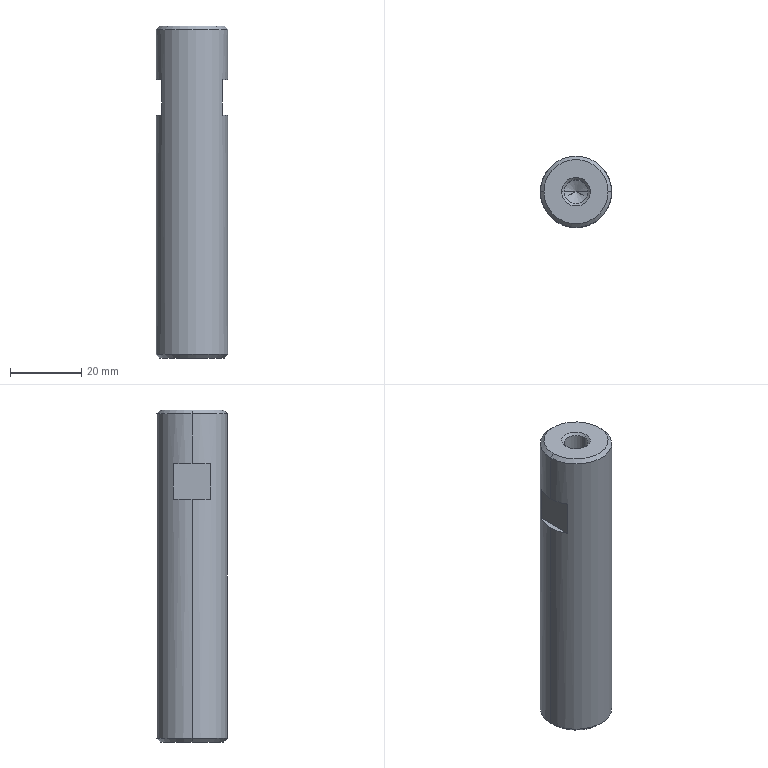Part | NX | features BREP 1 | 1 solid | 26 faces | box 20 x 20 x 93 mm | volume 27742 mm3 | cone 12 | plane 8 | cylinder 6 | commonest cylinder face diameters 6.647 x4 20 x2
STEP:
#1=CARTESIAN_POINT('',(3.324,0.,-92.323));
#2=VERTEX_POINT('',#1);
#3=CARTESIAN_POINT('',(-3.324,0.,-92.323));
#4=VERTEX_POINT('',#3);
#5=CARTESIAN_POINT('',(0.,0.,-92.323));
#6=DIRECTION('',(0.,0.,-1.));
#7=DIRECTION('',(-1.,0.,0.));
#8=AXIS2_PLACEMENT_3D('',#5,#6,#7);
#9=CIRCLE('',#8,3.324);
#10=EDGE_CURVE('',#2,#4,#9,.T.);
#11=ORIENTED_EDGE('',*,*,#10,.F.);
#12=CARTESIAN_POINT('',(4.,0.,-93.));
#13=VERTEX_POINT('',#12);
#14=CARTESIAN_POINT('',(4.,0.,-93.));
#15=DIRECTION('',(0.7071,0.,-0.7071));
#16=VECTOR('',#15,1000.);
#17=LINE('',#14,#16);
#18=EDGE_CURVE('',#13,#2,#17,.F.);
#19=ORIENTED_EDGE('',*,*,#18,.F.);
#20=CARTESIAN_POINT('',(-4.,0.,-93.));
#21=VERTEX_POINT('',#20);
#22=CARTESIAN_POINT('',(0.,0.,-93.));
#23=DIRECTION('',(0.,0.,-1.));
#24=DIRECTION('',(-1.,0.,0.));
#25=AXIS2_PLACEMENT_3D('',#22,#23,#24);
#26=CIRCLE('',#25,4.);
#27=EDGE_CURVE('',#13,#21,#26,.T.);
#28=ORIENTED_EDGE('',*,*,#27,.T.);
#29=CARTESIAN_POINT('',(-4.,0.,-93.));
#30=DIRECTION('',(-0.7071,0.,-0.7071));
#31=VECTOR('',#30,1000.);
#32=LINE('',#29,#31);
#33=EDGE_CURVE('',#21,#4,#32,.F.);
#34=ORIENTED_EDGE('',*,*,#33,.T.);
#35=EDGE_LOOP('',(#11,#19,#28,#34));
#36=FACE_BOUND('',#35,.T.);
#37=CARTESIAN_POINT('',(0.,0.,-93.));
#38=DIRECTION('',(0.,0.,-1.));
#39=DIRECTION('',(1.,0.,0.));
#40=AXIS2_PLACEMENT_3D('',#37,#38,#39);
#41=CONICAL_SURFACE('',#40,4.,0.7854);
#42=ADVANCED_FACE('',(#36),#41,.F.);
#43=CARTESIAN_POINT('',(3.324,0.,-76.5));
#44=VERTEX_POINT('',#43);
#45=CARTESIAN_POINT('',(-3.324,0.,-76.5));
#46=VERTEX_POINT('',#45);
#47=CARTESIAN_POINT('',(0.,0.,-76.5));
#48=DIRECTION('',(0.,0.,-1.));
#49=DIRECTION('',(-1.,0.,0.));
#50=AXIS2_PLACEMENT_3D('',#47,#48,#49);
#51=CIRCLE('',#50,3.324);
#52=EDGE_CURVE('',#44,#46,#51,.T.);
#53=ORIENTED_EDGE('',*,*,#52,.F.);
#54=CARTESIAN_POINT('',(3.324,0.,-93.));
#55=DIRECTION('',(0.,0.,-1.));
#56=VECTOR('',#55,1000.);
#57=LINE('',#54,#56);
#58=EDGE_CURVE('',#2,#44,#57,.F.);
#59=ORIENTED_EDGE('',*,*,#58,.F.);
#60=ORIENTED_EDGE('',*,*,#10,.T.);
#61=CARTESIAN_POINT('',(-3.324,0.,-93.));
#62=DIRECTION('',(0.,0.,-1.));
#63=VECTOR('',#62,1000.);
#64=LINE('',#61,#63);
#65=EDGE_CURVE('',#4,#46,#64,.F.);
#66=ORIENTED_EDGE('',*,*,#65,.T.);
#67=EDGE_LOOP('',(#53,#59,#60,#66));
#68=FACE_BOUND('',#67,.T.);
#69=CARTESIAN_POINT('',(0.,0.,-93.));
#70=DIRECTION('',(0.,0.,-1.));
#71=DIRECTION('',(1.,0.,0.));
#72=AXIS2_PLACEMENT_3D('',#69,#70,#71);
#73=CYLINDRICAL_SURFACE('',#72,3.324);
#74=ADVANCED_FACE('',(#68),#73,.F.);
#75=CARTESIAN_POINT('',(0.,0.,-74.581));
#76=VERTEX_POINT('',#75);
#77=CARTESIAN_POINT('',(-3.324,0.,-76.5));
#78=DIRECTION('',(-0.866,0.,-0.5));
#79=VECTOR('',#78,1000.);
#80=LINE('',#77,#79);
#81=EDGE_CURVE('',#46,#76,#80,.F.);
#82=ORIENTED_EDGE('',*,*,#81,.T.);
#83=CARTESIAN_POINT('',(3.324,0.,-76.5));
#84=DIRECTION('',(0.866,0.,-0.5));
#85=VECTOR('',#84,1000.);
#86=LINE('',#83,#85);
#87=EDGE_CURVE('',#44,#76,#86,.F.);
#88=ORIENTED_EDGE('',*,*,#87,.F.);
#89=ORIENTED_EDGE('',*,*,#52,.T.);
#90=EDGE_LOOP('',(#82,#88,#89));
#91=FACE_BOUND('',#90,.T.);
#92=CARTESIAN_POINT('',(0.,0.,-76.5));
#93=DIRECTION('',(0.,0.,-1.));
#94=DIRECTION('',(1.,0.,0.));
#95=AXIS2_PLACEMENT_3D('',#92,#93,#94);
#96=CONICAL_SURFACE('',#95,3.324,1.047);
#97=ADVANCED_FACE('',(#91),#96,.F.);
#98=CARTESIAN_POINT('',(-3.324,0.,-0.6765));
#99=VERTEX_POINT('',#98);
#100=CARTESIAN_POINT('',(3.324,0.,-0.6765));
#101=VERTEX_POINT('',#100);
#102=CARTESIAN_POINT('',(0.,0.,-0.6765));
#103=DIRECTION('',(0.,0.,1.));
#104=DIRECTION('',(1.,0.,0.));
#105=AXIS2_PLACEMENT_3D('',#102,#103,#104);
#106=CIRCLE('',#105,3.324);
#107=EDGE_CURVE('',#99,#101,#106,.T.);
#108=ORIENTED_EDGE('',*,*,#107,.F.);
#109=CARTESIAN_POINT('',(-4.,0.,0.));
#110=VERTEX_POINT('',#109);
#111=CARTESIAN_POINT('',(-4.,0.,0.));
#112=DIRECTION('',(-0.7071,0.,0.7071));
#113=VECTOR('',#112,1000.);
#114=LINE('',#111,#113);
#115=EDGE_CURVE('',#99,#110,#114,.T.);
#116=ORIENTED_EDGE('',*,*,#115,.T.);
#117=CARTESIAN_POINT('',(4.,0.,0.));
#118=VERTEX_POINT('',#117);
#119=CARTESIAN_POINT('',(0.,0.,0.));
#120=DIRECTION('',(0.,0.,1.));
#121=DIRECTION('',(1.,0.,0.));
#122=AXIS2_PLACEMENT_3D('',#119,#120,#121);
#123=CIRCLE('',#122,4.);
#124=EDGE_CURVE('',#110,#118,#123,.T.);
#125=ORIENTED_EDGE('',*,*,#124,.T.);
#126=CARTESIAN_POINT('',(4.,0.,0.));
#127=DIRECTION('',(0.7071,0.,0.7071));
#128=VECTOR('',#127,1000.);
#129=LINE('',#126,#128);
#130=EDGE_CURVE('',#101,#118,#129,.T.);
#131=ORIENTED_EDGE('',*,*,#130,.F.);
#132=EDGE_LOOP('',(#108,#116,#125,#131));
#133=FACE_BOUND('',#132,.T.);
#134=CARTESIAN_POINT('',(0.,0.,0.));
#135=DIRECTION('',(0.,0.,1.));
#136=DIRECTION('',(-1.,0.,0.));
#137=AXIS2_PLACEMENT_3D('',#134,#135,#136);
#138=CONICAL_SURFACE('',#137,4.,0.7854);
#139=ADVANCED_FACE('',(#133),#138,.F.);
#140=CARTESIAN_POINT('',(-3.324,0.,-16.5));
#141=VERTEX_POINT('',#140);
#142=CARTESIAN_POINT('',(3.324,0.,-16.5));
#143=VERTEX_POINT('',#142);
#144=CARTESIAN_POINT('',(0.,0.,-16.5));
#145=DIRECTION('',(0.,0.,1.));
#146=DIRECTION('',(1.,0.,0.));
#147=AXIS2_PLACEMENT_3D('',#144,#145,#146);
#148=CIRCLE('',#147,3.324);
#149=EDGE_CURVE('',#141,#143,#148,.T.);
#150=ORIENTED_EDGE('',*,*,#149,.F.);
#151=CARTESIAN_POINT('',(-3.324,0.,0.));
#152=DIRECTION('',(0.,0.,1.));
#153=VECTOR('',#152,1000.);
#154=LINE('',#151,#153);
#155=EDGE_CURVE('',#141,#99,#154,.T.);
#156=ORIENTED_EDGE('',*,*,#155,.T.);
#157=ORIENTED_EDGE('',*,*,#107,.T.);
#158=CARTESIAN_POINT('',(3.324,0.,0.));
#159=DIRECTION('',(0.,0.,1.));
#160=VECTOR('',#159,1000.);
#161=LINE('',#158,#160);
#162=EDGE_CURVE('',#143,#101,#161,.T.);
#163=ORIENTED_EDGE('',*,*,#162,.F.);
#164=EDGE_LOOP('',(#150,#156,#157,#163));
#165=FACE_BOUND('',#164,.T.);
#166=CARTESIAN_POINT('',(0.,0.,0.));
#167=DIRECTION('',(0.,0.,1.));
#168=DIRECTION('',(-1.,0.,0.));
#169=AXIS2_PLACEMENT_3D('',#166,#167,#168);
#170=CYLINDRICAL_SURFACE('',#169,3.324);
#171=ADVANCED_FACE('',(#165),#170,.F.);
#172=CARTESIAN_POINT('',(0.,0.,-18.419));
#173=VERTEX_POINT('',#172);
#174=CARTESIAN_POINT('',(3.324,0.,-16.5));
#175=DIRECTION('',(0.866,0.,0.5));
#176=VECTOR('',#175,1000.);
#177=LINE('',#174,#176);
#178=EDGE_CURVE('',#173,#143,#177,.T.);
#179=ORIENTED_EDGE('',*,*,#178,.F.);
#180=CARTESIAN_POINT('',(-3.324,0.,-16.5));
#181=DIRECTION('',(-0.866,0.,0.5));
#182=VECTOR('',#181,1000.);
#183=LINE('',#180,#182);
#184=EDGE_CURVE('',#173,#141,#183,.T.);
#185=ORIENTED_EDGE('',*,*,#184,.T.);
#186=ORIENTED_EDGE('',*,*,#149,.T.);
#187=EDGE_LOOP('',(#179,#185,#186));
#188=FACE_BOUND('',#187,.T.);
#189=CARTESIAN_POINT('',(0.,0.,-16.5));
#190=DIRECTION('',(0.,0.,1.));
#191=DIRECTION('',(-1.,0.,0.));
#192=AXIS2_PLACEMENT_3D('',#189,#190,#191);
#193=CONICAL_SURFACE('',#192,3.324,1.047);
#194=ADVANCED_FACE('',(#188),#193,.F.);
#195=CARTESIAN_POINT('',(9.,0.,-93.));
#196=VERTEX_POINT('',#195);
#197=CARTESIAN_POINT('',(-9.,0.,-93.));
#198=VERTEX_POINT('',#197);
#199=CARTESIAN_POINT('',(0.,0.,-93.));
#200=DIRECTION('',(0.,0.,1.));
#201=DIRECTION('',(1.,0.,0.));
#202=AXIS2_PLACEMENT_3D('',#199,#200,#201);
#203=CIRCLE('',#202,9.);
#204=EDGE_CURVE('',#196,#198,#203,.T.);
#205=ORIENTED_EDGE('',*,*,#204,.T.);
#206=CARTESIAN_POINT('',(-10.,0.,-92.));
#207=VERTEX_POINT('',#206);
#208=CARTESIAN_POINT('',(-9.,0.,-93.));
#209=DIRECTION('',(-0.7071,0.,0.7071));
#210=VECTOR('',#209,1000.);
#211=LINE('',#208,#210);
#212=EDGE_CURVE('',#198,#207,#211,.T.);
#213=ORIENTED_EDGE('',*,*,#212,.T.);
#214=CARTESIAN_POINT('',(10.,0.,-92.));
#215=VERTEX_POINT('',#214);
#216=CARTESIAN_POINT('',(0.,0.,-92.));
#217=DIRECTION('',(0.,0.,1.));
#218=DIRECTION('',(1.,0.,0.));
#219=AXIS2_PLACEMENT_3D('',#216,#217,#218);
#220=CIRCLE('',#219,10.);
#221=EDGE_CURVE('',#215,#207,#220,.T.);
#222=ORIENTED_EDGE('',*,*,#221,.F.);
#223=CARTESIAN_POINT('',(9.,0.,-93.));
#224=DIRECTION('',(0.7071,0.,0.7071));
#225=VECTOR('',#224,1000.);
#226=LINE('',#223,#225);
#227=EDGE_CURVE('',#196,#215,#226,.T.);
#228=ORIENTED_EDGE('',*,*,#227,.F.);
#229=EDGE_LOOP('',(#205,#213,#222,#228));
#230=FACE_BOUND('',#229,.T.);
#231=CARTESIAN_POINT('',(0.,0.,-93.));
#232=DIRECTION('',(0.,0.,1.));
#233=DIRECTION('',(-1.,0.,0.));
#234=AXIS2_PLACEMENT_3D('',#231,#232,#233);
#235=CONICAL_SURFACE('',#234,9.,0.7854);
#236=ADVANCED_FACE('',(#230),#235,.T.);
#237=CARTESIAN_POINT('',(9.,0.,0.));
#238=VERTEX_POINT('',#237);
#239=CARTESIAN_POINT('',(-9.,0.,0.));
#240=VERTEX_POINT('',#239);
#241=CARTESIAN_POINT('',(0.,0.,0.));
#242=DIRECTION('',(0.,0.,1.));
#243=DIRECTION('',(1.,0.,0.));
#244=AXIS2_PLACEMENT_3D('',#241,#242,#243);
#245=CIRCLE('',#244,9.);
#246=EDGE_CURVE('',#238,#240,#245,.T.);
#247=ORIENTED_EDGE('',*,*,#246,.F.);
#248=CARTESIAN_POINT('',(10.,0.,-1.));
#249=VERTEX_POINT('',#248);
#250=CARTESIAN_POINT('',(10.,0.,-1.));
#251=DIRECTION('',(0.7071,0.,-0.7071));
#252=VECTOR('',#251,1000.);
#253=LINE('',#250,#252);
#254=EDGE_CURVE('',#249,#238,#253,.F.);
#255=ORIENTED_EDGE('',*,*,#254,.F.);
#256=CARTESIAN_POINT('',(-10.,0.,-1.));
#257=VERTEX_POINT('',#256);
#258=CARTESIAN_POINT('',(0.,0.,-1.));
#259=DIRECTION('',(0.,0.,1.));
#260=DIRECTION('',(1.,0.,0.));
#261=AXIS2_PLACEMENT_3D('',#258,#259,#260);
#262=CIRCLE('',#261,10.);
#263=EDGE_CURVE('',#249,#257,#262,.T.);
#264=ORIENTED_EDGE('',*,*,#263,.T.);
#265=CARTESIAN_POINT('',(-10.,0.,-1.));
#266=DIRECTION('',(-0.7071,0.,-0.7071));
#267=VECTOR('',#266,1000.);
#268=LINE('',#265,#267);
#269=EDGE_CURVE('',#257,#240,#268,.F.);
#270=ORIENTED_EDGE('',*,*,#269,.T.);
#271=EDGE_LOOP('',(#247,#255,#264,#270));
#272=FACE_BOUND('',#271,.T.);
#273=CARTESIAN_POINT('',(0.,0.,-1.));
#274=DIRECTION('',(0.,0.,-1.));
#275=DIRECTION('',(1.,0.,0.));
#276=AXIS2_PLACEMENT_3D('',#273,#274,#275);
#277=CONICAL_SURFACE('',#276,10.,0.7854);
#278=ADVANCED_FACE('',(#272),#277,.T.);
#279=ORIENTED_EDGE('',*,*,#221,.T.);
#280=CARTESIAN_POINT('',(-10.,0.,-25.));
#281=VERTEX_POINT('',#280);
#282=CARTESIAN_POINT('',(-10.,0.,-93.));
#283=DIRECTION('',(0.,0.,1.));
#284=VECTOR('',#283,1000.);
#285=LINE('',#282,#284);
#286=EDGE_CURVE('',#207,#281,#285,.T.);
#287=ORIENTED_EDGE('',*,*,#286,.T.);
#288=CARTESIAN_POINT('',(-8.5,5.268,-25.));
#289=VERTEX_POINT('',#288);
#290=CARTESIAN_POINT('',(0.,0.,-25.));
#291=DIRECTION('',(0.,0.,1.));
#292=DIRECTION('',(1.,0.,0.));
#293=AXIS2_PLACEMENT_3D('',#290,#291,#292);
#294=CIRCLE('',#293,10.);
#295=EDGE_CURVE('',#289,#281,#294,.T.);
#296=ORIENTED_EDGE('',*,*,#295,.F.);
#297=CARTESIAN_POINT('',(-8.5,5.268,-15.));
#298=VERTEX_POINT('',#297);
#299=CARTESIAN_POINT('',(-8.5,5.268,-25.));
#300=DIRECTION('',(0.,0.,1.));
#301=VECTOR('',#300,1000.);
#302=LINE('',#299,#301);
#303=EDGE_CURVE('',#289,#298,#302,.T.);
#304=ORIENTED_EDGE('',*,*,#303,.T.);
#305=CARTESIAN_POINT('',(-10.,0.,-15.));
#306=VERTEX_POINT('',#305);
#307=CARTESIAN_POINT('',(0.,0.,-15.));
#308=DIRECTION('',(0.,0.,1.));
#309=DIRECTION('',(1.,0.,0.));
#310=AXIS2_PLACEMENT_3D('',#307,#308,#309);
#311=CIRCLE('',#310,10.);
#312=EDGE_CURVE('',#298,#306,#311,.T.);
#313=ORIENTED_EDGE('',*,*,#312,.T.);
#314=CARTESIAN_POINT('',(-10.,0.,-93.));
#315=DIRECTION('',(0.,0.,1.));
#316=VECTOR('',#315,1000.);
#317=LINE('',#314,#316);
#318=EDGE_CURVE('',#306,#257,#317,.T.);
#319=ORIENTED_EDGE('',*,*,#318,.T.);
#320=ORIENTED_EDGE('',*,*,#263,.F.);
#321=CARTESIAN_POINT('',(10.,0.,-15.));
#322=VERTEX_POINT('',#321);
#323=CARTESIAN_POINT('',(10.,0.,-93.));
#324=DIRECTION('',(0.,0.,1.));
#325=VECTOR('',#324,1000.);
#326=LINE('',#323,#325);
#327=EDGE_CURVE('',#322,#249,#326,.T.);
#328=ORIENTED_EDGE('',*,*,#327,.F.);
#329=CARTESIAN_POINT('',(8.5,5.268,-15.));
#330=VERTEX_POINT('',#329);
#331=CARTESIAN_POINT('',(0.,0.,-15.));
#332=DIRECTION('',(0.,0.,1.));
#333=DIRECTION('',(1.,0.,0.));
#334=AXIS2_PLACEMENT_3D('',#331,#332,#333);
#335=CIRCLE('',#334,10.);
#336=EDGE_CURVE('',#322,#330,#335,.T.);
#337=ORIENTED_EDGE('',*,*,#336,.T.);
#338=CARTESIAN_POINT('',(8.5,5.268,-25.));
#339=VERTEX_POINT('',#338);
#340=CARTESIAN_POINT('',(8.5,5.268,-25.));
#341=DIRECTION('',(0.,0.,1.));
#342=VECTOR('',#341,1000.);
#343=LINE('',#340,#342);
#344=EDGE_CURVE('',#339,#330,#343,.T.);
#345=ORIENTED_EDGE('',*,*,#344,.F.);
#346=CARTESIAN_POINT('',(10.,0.,-25.));
#347=VERTEX_POINT('',#346);
#348=CARTESIAN_POINT('',(0.,0.,-25.));
#349=DIRECTION('',(0.,0.,1.));
#350=DIRECTION('',(1.,0.,0.));
#351=AXIS2_PLACEMENT_3D('',#348,#349,#350);
#352=CIRCLE('',#351,10.);
#353=EDGE_CURVE('',#347,#339,#352,.T.);
#354=ORIENTED_EDGE('',*,*,#353,.F.);
#355=CARTESIAN_POINT('',(10.,0.,-93.));
#356=DIRECTION('',(0.,0.,1.));
#357=VECTOR('',#356,1000.);
#358=LINE('',#355,#357);
#359=EDGE_CURVE('',#215,#347,#358,.T.);
#360=ORIENTED_EDGE('',*,*,#359,.F.);
#361=EDGE_LOOP('',(#279,#287,#296,#304,#313,#319,#320,#328,#337,#345,#354,#360));
#362=FACE_BOUND('',#361,.T.);
#363=CARTESIAN_POINT('',(0.,0.,-93.));
#364=DIRECTION('',(0.,0.,1.));
#365=DIRECTION('',(-1.,0.,0.));
#366=AXIS2_PLACEMENT_3D('',#363,#364,#365);
#367=CYLINDRICAL_SURFACE('',#366,10.);
#368=ADVANCED_FACE('',(#362),#367,.T.);
#369=ORIENTED_EDGE('',*,*,#286,.F.);
#370=CARTESIAN_POINT('',(0.,0.,-92.));
#371=DIRECTION('',(0.,0.,1.));
#372=DIRECTION('',(1.,0.,0.));
#373=AXIS2_PLACEMENT_3D('',#370,#371,#372);
#374=CIRCLE('',#373,10.);
#375=EDGE_CURVE('',#207,#215,#374,.T.);
#376=ORIENTED_EDGE('',*,*,#375,.T.);
#377=ORIENTED_EDGE('',*,*,#359,.T.);
#378=CARTESIAN_POINT('',(8.5,-5.268,-25.));
#379=VERTEX_POINT('',#378);
#380=CARTESIAN_POINT('',(0.,0.,-25.));
#381=DIRECTION('',(0.,0.,1.));
#382=DIRECTION('',(1.,0.,0.));
#383=AXIS2_PLACEMENT_3D('',#380,#381,#382);
#384=CIRCLE('',#383,10.);
#385=EDGE_CURVE('',#379,#347,#384,.T.);
#386=ORIENTED_EDGE('',*,*,#385,.F.);
#387=CARTESIAN_POINT('',(8.5,-5.268,-15.));
#388=VERTEX_POINT('',#387);
#389=CARTESIAN_POINT('',(8.5,-5.268,-25.));
#390=DIRECTION('',(0.,0.,1.));
#391=VECTOR('',#390,1000.);
#392=LINE('',#389,#391);
#393=EDGE_CURVE('',#379,#388,#392,.T.);
#394=ORIENTED_EDGE('',*,*,#393,.T.);
#395=CARTESIAN_POINT('',(0.,0.,-15.));
#396=DIRECTION('',(0.,0.,1.));
#397=DIRECTION('',(1.,0.,0.));
#398=AXIS2_PLACEMENT_3D('',#395,#396,#397);
#399=CIRCLE('',#398,10.);
#400=EDGE_CURVE('',#388,#322,#399,.T.);
#401=ORIENTED_EDGE('',*,*,#400,.T.);
#402=ORIENTED_EDGE('',*,*,#327,.T.);
#403=CARTESIAN_POINT('',(0.,0.,-1.));
#404=DIRECTION('',(0.,0.,1.));
#405=DIRECTION('',(1.,0.,0.));
#406=AXIS2_PLACEMENT_3D('',#403,#404,#405);
#407=CIRCLE('',#406,10.);
#408=EDGE_CURVE('',#257,#249,#407,.T.);
#409=ORIENTED_EDGE('',*,*,#408,.F.);
#410=ORIENTED_EDGE('',*,*,#318,.F.);
#411=CARTESIAN_POINT('',(-8.5,-5.268,-15.));
#412=VERTEX_POINT('',#411);
#413=CARTESIAN_POINT('',(0.,0.,-15.));
#414=DIRECTION('',(0.,0.,1.));
#415=DIRECTION('',(1.,0.,0.));
#416=AXIS2_PLACEMENT_3D('',#413,#414,#415);
#417=CIRCLE('',#416,10.);
#418=EDGE_CURVE('',#306,#412,#417,.T.);
#419=ORIENTED_EDGE('',*,*,#418,.T.);
#420=CARTESIAN_POINT('',(-8.5,-5.268,-25.));
#421=VERTEX_POINT('',#420);
#422=CARTESIAN_POINT('',(-8.5,-5.268,-25.));
#423=DIRECTION('',(0.,0.,1.));
#424=VECTOR('',#423,1000.);
#425=LINE('',#422,#424);
#426=EDGE_CURVE('',#421,#412,#425,.T.);
#427=ORIENTED_EDGE('',*,*,#426,.F.);
#428=CARTESIAN_POINT('',(0.,0.,-25.));
#429=DIRECTION('',(0.,0.,1.));
#430=DIRECTION('',(1.,0.,0.));
#431=AXIS2_PLACEMENT_3D('',#428,#429,#430);
#432=CIRCLE('',#431,10.);
#433=EDGE_CURVE('',#281,#421,#432,.T.);
#434=ORIENTED_EDGE('',*,*,#433,.F.);
#435=EDGE_LOOP('',(#369,#376,#377,#386,#394,#401,#402,#409,#410,#419,#427,#434));
#436=FACE_BOUND('',#435,.T.);
#437=CARTESIAN_POINT('',(0.,0.,-93.));
#438=DIRECTION('',(0.,0.,1.));
#439=DIRECTION('',(-1.,0.,0.));
#440=AXIS2_PLACEMENT_3D('',#437,#438,#439);
#441=CYLINDRICAL_SURFACE('',#440,10.);
#442=ADVANCED_FACE('',(#436),#441,.T.);
#443=CARTESIAN_POINT('',(0.,0.,0.));
#444=DIRECTION('',(0.,0.,1.));
#445=DIRECTION('',(1.,0.,0.));
#446=AXIS2_PLACEMENT_3D('',#443,#444,#445);
#447=CIRCLE('',#446,4.);
#448=EDGE_CURVE('',#118,#110,#447,.T.);
#449=ORIENTED_EDGE('',*,*,#448,.F.);
#450=ORIENTED_EDGE('',*,*,#124,.F.);
#451=EDGE_LOOP('',(#449,#450));
#452=FACE_BOUND('',#451,.T.);
#453=CARTESIAN_POINT('',(0.,0.,0.));
#454=DIRECTION('',(0.,0.,1.));
#455=DIRECTION('',(1.,0.,0.));
#456=AXIS2_PLACEMENT_3D('',#453,#454,#455);
#457=CIRCLE('',#456,9.);
#458=EDGE_CURVE('',#240,#238,#457,.T.);
#459=ORIENTED_EDGE('',*,*,#458,.T.);
#460=ORIENTED_EDGE('',*,*,#246,.T.);
#461=EDGE_LOOP('',(#459,#460));
#462=FACE_BOUND('',#461,.T.);
#463=CARTESIAN_POINT('',(0.,0.,0.));
#464=DIRECTION('',(0.,0.,-1.));
#465=DIRECTION('',(1.,0.,0.));
#466=AXIS2_PLACEMENT_3D('',#463,#464,#465);
#467=PLANE('',#466);
#468=ADVANCED_FACE('',(#452,#462),#467,.F.);
#469=ORIENTED_EDGE('',*,*,#254,.T.);
#470=ORIENTED_EDGE('',*,*,#458,.F.);
#471=ORIENTED_EDGE('',*,*,#269,.F.);
#472=ORIENTED_EDGE('',*,*,#408,.T.);
#473=EDGE_LOOP('',(#469,#470,#471,#472));
#474=FACE_BOUND('',#473,.T.);
#475=CARTESIAN_POINT('',(0.,0.,-1.));
#476=DIRECTION('',(0.,0.,-1.));
#477=DIRECTION('',(1.,0.,0.));
#478=AXIS2_PLACEMENT_3D('',#475,#476,#477);
#479=CONICAL_SURFACE('',#478,10.,0.7854);
#480=ADVANCED_FACE('',(#474),#479,.T.);
#481=ORIENTED_EDGE('',*,*,#212,.F.);
#482=CARTESIAN_POINT('',(0.,0.,-93.));
#483=DIRECTION('',(0.,0.,1.));
#484=DIRECTION('',(1.,0.,0.));
#485=AXIS2_PLACEMENT_3D('',#482,#483,#484);
#486=CIRCLE('',#485,9.);
#487=EDGE_CURVE('',#198,#196,#486,.T.);
#488=ORIENTED_EDGE('',*,*,#487,.T.);
#489=ORIENTED_EDGE('',*,*,#227,.T.);
#490=ORIENTED_EDGE('',*,*,#375,.F.);
#491=EDGE_LOOP('',(#481,#488,#489,#490));
#492=FACE_BOUND('',#491,.T.);
#493=CARTESIAN_POINT('',(0.,0.,-93.));
#494=DIRECTION('',(0.,0.,1.));
#495=DIRECTION('',(-1.,0.,0.));
#496=AXIS2_PLACEMENT_3D('',#493,#494,#495);
#497=CONICAL_SURFACE('',#496,9.,0.7854);
#498=ADVANCED_FACE('',(#492),#497,.T.);
#499=CARTESIAN_POINT('',(0.,0.,-93.));
#500=DIRECTION('',(0.,0.,-1.));
#501=DIRECTION('',(-1.,0.,0.));
#502=AXIS2_PLACEMENT_3D('',#499,#500,#501);
#503=CIRCLE('',#502,4.);
#504=EDGE_CURVE('',#21,#13,#503,.T.);
#505=ORIENTED_EDGE('',*,*,#504,.F.);
#506=ORIENTED_EDGE('',*,*,#27,.F.);
#507=EDGE_LOOP('',(#505,#506));
#508=FACE_BOUND('',#507,.T.);
#509=ORIENTED_EDGE('',*,*,#204,.F.);
#510=ORIENTED_EDGE('',*,*,#487,.F.);
#511=EDGE_LOOP('',(#509,#510));
#512=FACE_BOUND('',#511,.T.);
#513=CARTESIAN_POINT('',(0.,9.,-93.));
#514=DIRECTION('',(0.,0.,1.));
#515=DIRECTION('',(-1.,0.,0.));
#516=AXIS2_PLACEMENT_3D('',#513,#514,#515);
#517=PLANE('',#516);
#518=ADVANCED_FACE('',(#508,#512),#517,.F.);
#519=ORIENTED_EDGE('',*,*,#184,.F.);
#520=ORIENTED_EDGE('',*,*,#178,.T.);
#521=CARTESIAN_POINT('',(0.,0.,-16.5));
#522=DIRECTION('',(0.,0.,1.));
#523=DIRECTION('',(1.,0.,0.));
#524=AXIS2_PLACEMENT_3D('',#521,#522,#523);
#525=CIRCLE('',#524,3.324);
#526=EDGE_CURVE('',#143,#141,#525,.T.);
#527=ORIENTED_EDGE('',*,*,#526,.T.);
#528=EDGE_LOOP('',(#519,#520,#527));
#529=FACE_BOUND('',#528,.T.);
#530=CARTESIAN_POINT('',(0.,0.,-16.5));
#531=DIRECTION('',(0.,0.,1.));
#532=DIRECTION('',(-1.,0.,0.));
#533=AXIS2_PLACEMENT_3D('',#530,#531,#532);
#534=CONICAL_SURFACE('',#533,3.324,1.047);
#535=ADVANCED_FACE('',(#529),#534,.F.);
#536=ORIENTED_EDGE('',*,*,#155,.F.);
#537=ORIENTED_EDGE('',*,*,#526,.F.);
#538=ORIENTED_EDGE('',*,*,#162,.T.);
#539=CARTESIAN_POINT('',(0.,0.,-0.6765));
#540=DIRECTION('',(0.,0.,1.));
#541=DIRECTION('',(1.,0.,0.));
#542=AXIS2_PLACEMENT_3D('',#539,#540,#541);
#543=CIRCLE('',#542,3.324);
#544=EDGE_CURVE('',#101,#99,#543,.T.);
#545=ORIENTED_EDGE('',*,*,#544,.T.);
#546=EDGE_LOOP('',(#536,#537,#538,#545));
#547=FACE_BOUND('',#546,.T.);
#548=CARTESIAN_POINT('',(0.,0.,0.));
#549=DIRECTION('',(0.,0.,1.));
#550=DIRECTION('',(-1.,0.,0.));
#551=AXIS2_PLACEMENT_3D('',#548,#549,#550);
#552=CYLINDRICAL_SURFACE('',#551,3.324);
#553=ADVANCED_FACE('',(#547),#552,.F.);
#554=ORIENTED_EDGE('',*,*,#115,.F.);
#555=ORIENTED_EDGE('',*,*,#544,.F.);
#556=ORIENTED_EDGE('',*,*,#130,.T.);
#557=ORIENTED_EDGE('',*,*,#448,.T.);
#558=EDGE_LOOP('',(#554,#555,#556,#557));
#559=FACE_BOUND('',#558,.T.);
#560=CARTESIAN_POINT('',(0.,0.,0.));
#561=DIRECTION('',(0.,0.,1.));
#562=DIRECTION('',(-1.,0.,0.));
#563=AXIS2_PLACEMENT_3D('',#560,#561,#562);
#564=CONICAL_SURFACE('',#563,4.,0.7854);
#565=ADVANCED_FACE('',(#559),#564,.F.);
#566=ORIENTED_EDGE('',*,*,#87,.T.);
#567=ORIENTED_EDGE('',*,*,#81,.F.);
#568=CARTESIAN_POINT('',(0.,0.,-76.5));
#569=DIRECTION('',(0.,0.,-1.));
#570=DIRECTION('',(-1.,0.,0.));
#571=AXIS2_PLACEMENT_3D('',#568,#569,#570);
#572=CIRCLE('',#571,3.324);
#573=EDGE_CURVE('',#46,#44,#572,.T.);
#574=ORIENTED_EDGE('',*,*,#573,.T.);
#575=EDGE_LOOP('',(#566,#567,#574));
#576=FACE_BOUND('',#575,.T.);
#577=CARTESIAN_POINT('',(0.,0.,-76.5));
#578=DIRECTION('',(0.,0.,-1.));
#579=DIRECTION('',(1.,0.,0.));
#580=AXIS2_PLACEMENT_3D('',#577,#578,#579);
#581=CONICAL_SURFACE('',#580,3.324,1.047);
#582=ADVANCED_FACE('',(#576),#581,.F.);
#583=ORIENTED_EDGE('',*,*,#58,.T.);
#584=ORIENTED_EDGE('',*,*,#573,.F.);
#585=ORIENTED_EDGE('',*,*,#65,.F.);
#586=CARTESIAN_POINT('',(0.,0.,-92.323));
#587=DIRECTION('',(0.,0.,-1.));
#588=DIRECTION('',(-1.,0.,0.));
#589=AXIS2_PLACEMENT_3D('',#586,#587,#588);
#590=CIRCLE('',#589,3.324);
#591=EDGE_CURVE('',#4,#2,#590,.T.);
#592=ORIENTED_EDGE('',*,*,#591,.T.);
#593=EDGE_LOOP('',(#583,#584,#585,#592));
#594=FACE_BOUND('',#593,.T.);
#595=CARTESIAN_POINT('',(0.,0.,-93.));
#596=DIRECTION('',(0.,0.,-1.));
#597=DIRECTION('',(1.,0.,0.));
#598=AXIS2_PLACEMENT_3D('',#595,#596,#597);
#599=CYLINDRICAL_SURFACE('',#598,3.324);
#600=ADVANCED_FACE('',(#594),#599,.F.);
#601=ORIENTED_EDGE('',*,*,#18,.T.);
#602=ORIENTED_EDGE('',*,*,#591,.F.);
#603=ORIENTED_EDGE('',*,*,#33,.F.);
#604=ORIENTED_EDGE('',*,*,#504,.T.);
#605=EDGE_LOOP('',(#601,#602,#603,#604));
#606=FACE_BOUND('',#605,.T.);
#607=CARTESIAN_POINT('',(0.,0.,-93.));
#608=DIRECTION('',(0.,0.,-1.));
#609=DIRECTION('',(1.,0.,0.));
#610=AXIS2_PLACEMENT_3D('',#607,#608,#609);
#611=CONICAL_SURFACE('',#610,4.,0.7854);
#612=ADVANCED_FACE('',(#606),#611,.F.);
#613=CARTESIAN_POINT('',(-8.5,5.268,-15.));
#614=DIRECTION('',(0.,-1.,0.));
#615=VECTOR('',#614,1000.);
#616=LINE('',#613,#615);
#617=EDGE_CURVE('',#298,#412,#616,.T.);
#618=ORIENTED_EDGE('',*,*,#617,.F.);
#619=ORIENTED_EDGE('',*,*,#303,.F.);
#620=CARTESIAN_POINT('',(-8.5,5.268,-25.));
#621=DIRECTION('',(0.,-1.,0.));
#622=VECTOR('',#621,1000.);
#623=LINE('',#620,#622);
#624=EDGE_CURVE('',#289,#421,#623,.T.);
#625=ORIENTED_EDGE('',*,*,#624,.T.);
#626=ORIENTED_EDGE('',*,*,#426,.T.);
#627=EDGE_LOOP('',(#618,#619,#625,#626));
#628=FACE_BOUND('',#627,.T.);
#629=CARTESIAN_POINT('',(-8.5,5.268,-25.));
#630=DIRECTION('',(-1.,0.,0.));
#631=DIRECTION('',(0.,0.,-1.));
#632=AXIS2_PLACEMENT_3D('',#629,#630,#631);
#633=PLANE('',#632);
#634=ADVANCED_FACE('',(#628),#633,.T.);
#635=ORIENTED_EDGE('',*,*,#617,.T.);
#636=ORIENTED_EDGE('',*,*,#418,.F.);
#637=ORIENTED_EDGE('',*,*,#312,.F.);
#638=EDGE_LOOP('',(#635,#636,#637));
#639=FACE_BOUND('',#638,.T.);
#640=CARTESIAN_POINT('',(0.,0.,-15.));
#641=DIRECTION('',(0.,0.,1.));
#642=DIRECTION('',(-1.,0.,0.));
#643=AXIS2_PLACEMENT_3D('',#640,#641,#642);
#644=PLANE('',#643);
#645=ADVANCED_FACE('',(#639),#644,.F.);
#646=ORIENTED_EDGE('',*,*,#295,.T.);
#647=ORIENTED_EDGE('',*,*,#433,.T.);
#648=ORIENTED_EDGE('',*,*,#624,.F.);
#649=EDGE_LOOP('',(#646,#647,#648));
#650=FACE_BOUND('',#649,.T.);
#651=CARTESIAN_POINT('',(0.,0.,-25.));
#652=DIRECTION('',(0.,0.,1.));
#653=DIRECTION('',(-1.,0.,0.));
#654=AXIS2_PLACEMENT_3D('',#651,#652,#653);
#655=PLANE('',#654);
#656=ADVANCED_FACE('',(#650),#655,.T.);
#657=ORIENTED_EDGE('',*,*,#385,.T.);
#658=ORIENTED_EDGE('',*,*,#353,.T.);
#659=CARTESIAN_POINT('',(8.5,-5.268,-25.));
#660=DIRECTION('',(0.,1.,0.));
#661=VECTOR('',#660,1000.);
#662=LINE('',#659,#661);
#663=EDGE_CURVE('',#379,#339,#662,.T.);
#664=ORIENTED_EDGE('',*,*,#663,.F.);
#665=EDGE_LOOP('',(#657,#658,#664));
#666=FACE_BOUND('',#665,.T.);
#667=CARTESIAN_POINT('',(0.,0.,-25.));
#668=DIRECTION('',(0.,0.,1.));
#669=DIRECTION('',(-1.,0.,0.));
#670=AXIS2_PLACEMENT_3D('',#667,#668,#669);
#671=PLANE('',#670);
#672=ADVANCED_FACE('',(#666),#671,.T.);
#673=CARTESIAN_POINT('',(8.5,-5.268,-15.));
#674=DIRECTION('',(0.,1.,0.));
#675=VECTOR('',#674,1000.);
#676=LINE('',#673,#675);
#677=EDGE_CURVE('',#388,#330,#676,.T.);
#678=ORIENTED_EDGE('',*,*,#677,.T.);
#679=ORIENTED_EDGE('',*,*,#336,.F.);
#680=ORIENTED_EDGE('',*,*,#400,.F.);
#681=EDGE_LOOP('',(#678,#679,#680));
#682=FACE_BOUND('',#681,.T.);
#683=CARTESIAN_POINT('',(0.,0.,-15.));
#684=DIRECTION('',(0.,0.,1.));
#685=DIRECTION('',(-1.,0.,0.));
#686=AXIS2_PLACEMENT_3D('',#683,#684,#685);
#687=PLANE('',#686);
#688=ADVANCED_FACE('',(#682),#687,.F.);
#689=ORIENTED_EDGE('',*,*,#677,.F.);
#690=ORIENTED_EDGE('',*,*,#393,.F.);
#691=ORIENTED_EDGE('',*,*,#663,.T.);
#692=ORIENTED_EDGE('',*,*,#344,.T.);
#693=EDGE_LOOP('',(#689,#690,#691,#692));
#694=FACE_BOUND('',#693,.T.);
#695=CARTESIAN_POINT('',(8.5,-5.268,-25.));
#696=DIRECTION('',(1.,0.,0.));
#697=DIRECTION('',(0.,0.,1.));
#698=AXIS2_PLACEMENT_3D('',#695,#696,#697);
#699=PLANE('',#698);
#700=ADVANCED_FACE('',(#694),#699,.T.);
#701=CLOSED_SHELL('',(#42,#74,#97,#139,#171,#194,#236,#278,#368,#442,#468,#480,#498,#518,#535,#553,#565,#582,#600,#612,#634,#645,#656,#672,#688,#700));
#702=MANIFOLD_SOLID_BREP('',#701);
#703=(LENGTH_UNIT()NAMED_UNIT(*)SI_UNIT(.MILLI.,.METRE.));
#704=UNCERTAINTY_MEASURE_WITH_UNIT(LENGTH_MEASURE(0.00001),#703,'','');
#705=(NAMED_UNIT(*)PLANE_ANGLE_UNIT()SI_UNIT($,.RADIAN.));
#706=(NAMED_UNIT(*)SI_UNIT($,.STERADIAN.)SOLID_ANGLE_UNIT());
#707=(GEOMETRIC_REPRESENTATION_CONTEXT(3)GLOBAL_UNCERTAINTY_ASSIGNED_CONTEXT((#704))GLOBAL_UNIT_ASSIGNED_CONTEXT((#703,#705,#706))REPRESENTATION_CONTEXT('',''));
#708=ADVANCED_BREP_SHAPE_REPRESENTATION('',(#702),#707);